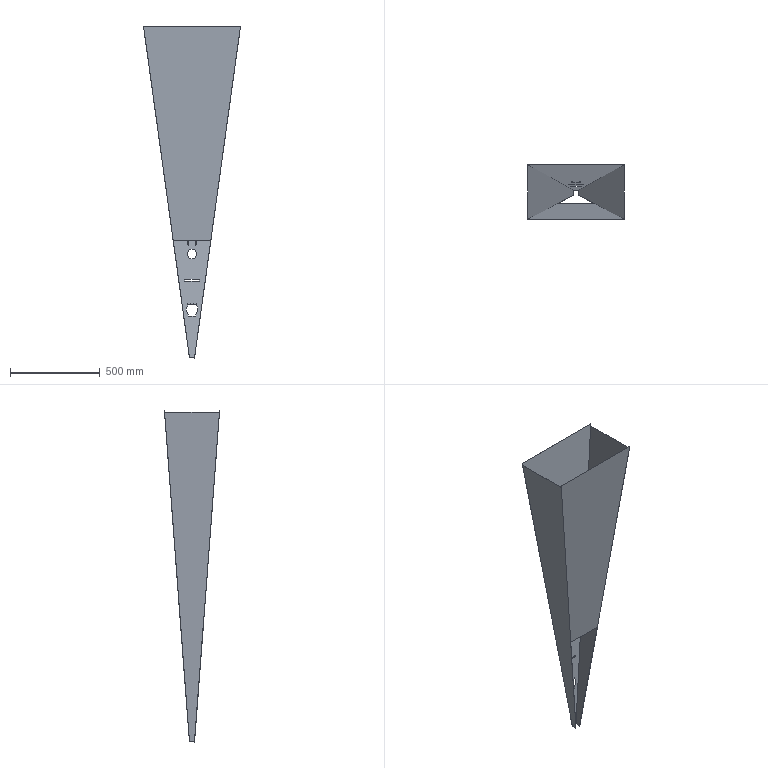Part | SolidWorks | features BaseBody 1 | 1 solid | 52 faces | box 540.73 x 307.803 x 1849 mm | volume 794159 mm3 | plane 34 | cylinder 10 | spline 8 | commonest cylinder face diameters 4 x6 52.593 x2 65 x2